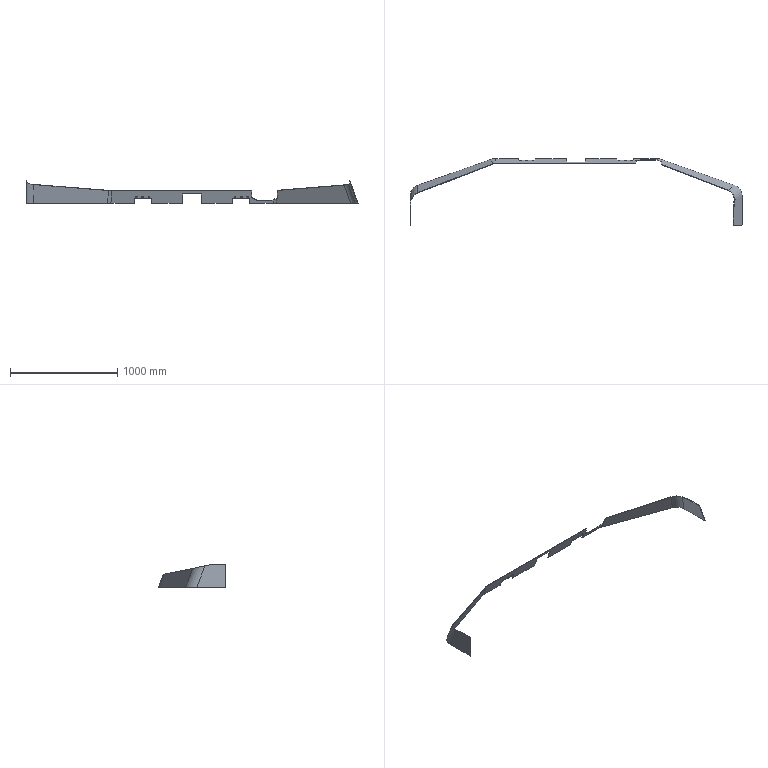Part | STEP file | 4A2-54-11L11_1 | 1 solid | 88 faces | box 3098 x 622.4 x 213.7 mm | volume 2346109 mm3 | plane 42 | cylinder 38 | spline 8 | commonest cylinder face diameters 10 x12 15 x12 20 x4 200 x4 209 x4 12 x2